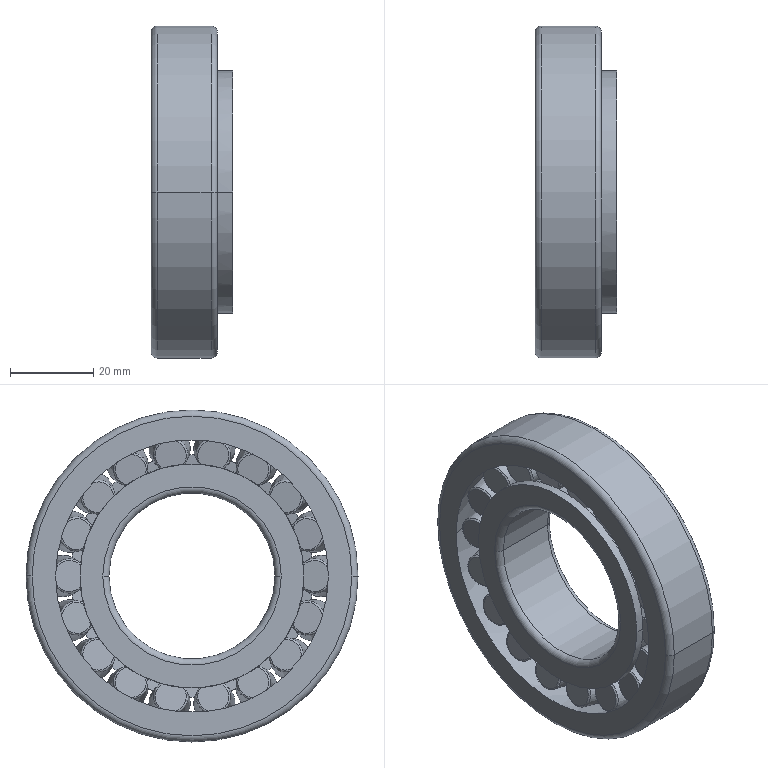Part | SolidWorks | features Revolution 3, CirPattern 1 | 1 solid | 172 faces | box 19.75 x 80 x 80 mm | volume 50008 mm3 | torus 80 | cone 44 | plane 40 | cylinder 8 | commonest cylinder face diameters 40 x2 53.964 x2 58.443 x2 80 x2